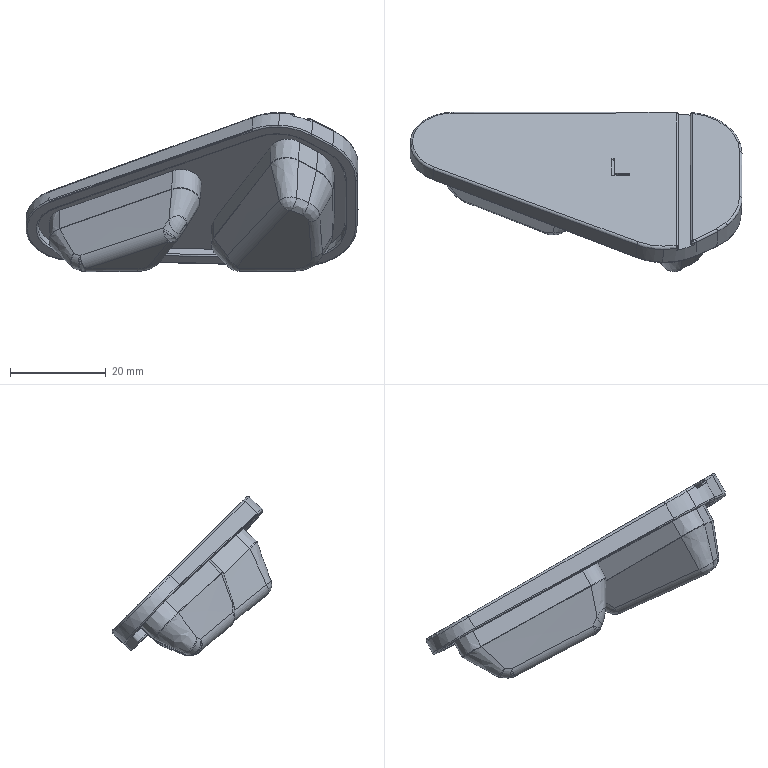Part | SolidWorks | features BaseBody 1 | 1 solid | 156 faces | box 69.595 x 33.418 x 33.337 mm | volume 16534 mm3 | spline 47 | cylinder 44 | plane 32 | sphere 15 | torus 13 | cone 5 | commonest cylinder face diameters 0.6 x16 1 x11 5 x3 19.026 x3 24.024 x2 5.004 x1